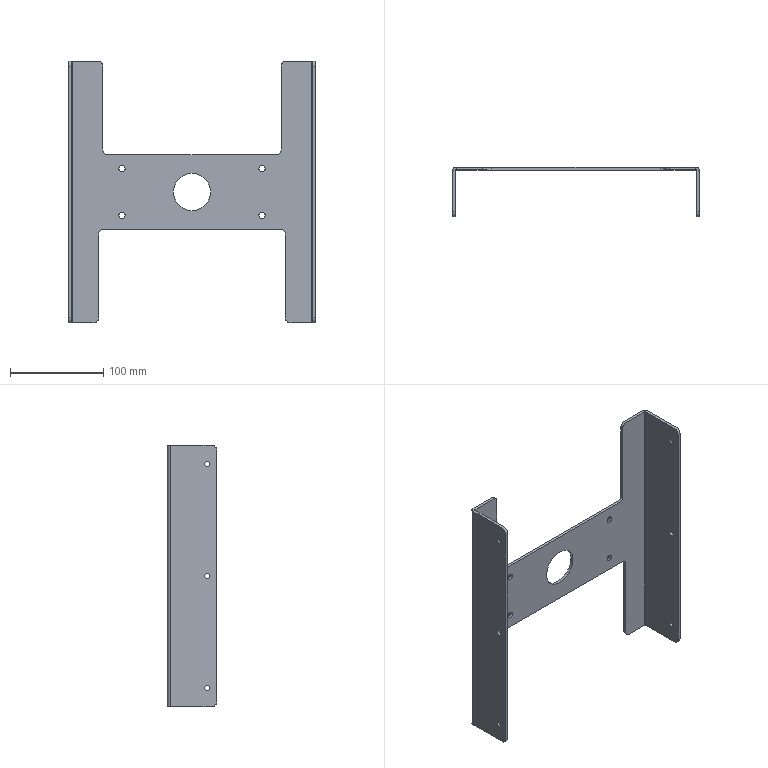Part | SolidWorks | features HoleWzd 2, ICE 2, Fillet 1, FlatPattern 1, SMBaseFlange 1, SheetMetal 1 | 1 solid | 64 faces | box 264.5 x 53 x 280 mm | volume 182601 mm3 | cylinder 38 | plane 26 | commonest cylinder face diameters 5.5 x12 10 x12 6.6 x8 1.473 x2 7.473 x2 40 x2